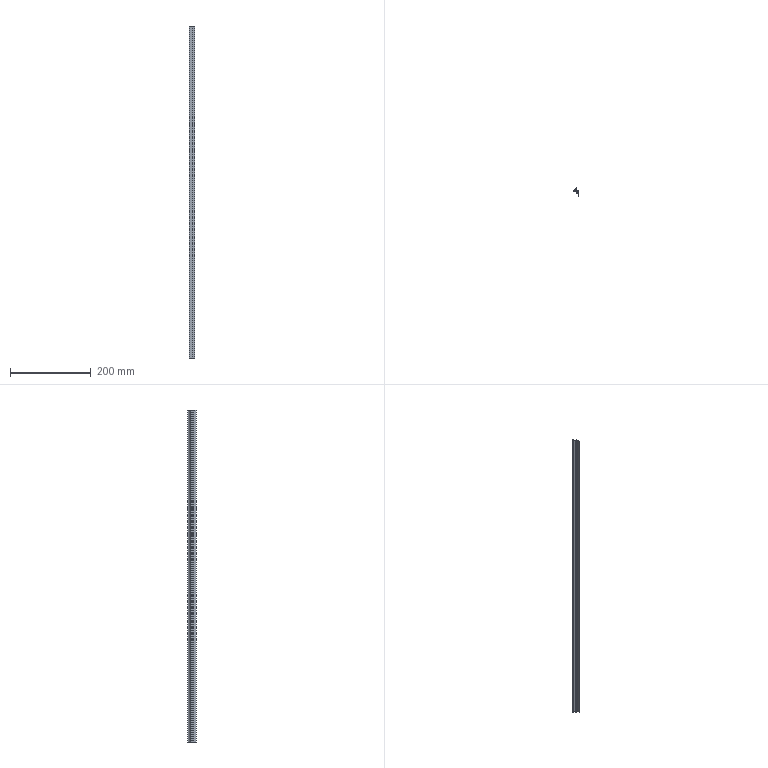Part | SolidWorks | features BaseBody 1, ICE 1, MoveFace 1 | 1 solid | 27 faces | box 14 x 20.3 x 820 mm | volume 41751 mm3 | plane 20 | cylinder 7 | commonest cylinder face diameters 0.387 x2 0.8 x2 0.4 x1 20 x1 22 x1
STEP:
#1=CARTESIAN_POINT('',(-5.304,-0.625,200.));
#2=VERTEX_POINT('',#1);
#3=CARTESIAN_POINT('',(-5.449,-0.8125,200.));
#4=VERTEX_POINT('',#3);
#5=CARTESIAN_POINT('',(-5.255,-0.8125,200.));
#6=DIRECTION('',(0.,0.,1.));
#7=DIRECTION('',(-1.,0.,0.));
#8=AXIS2_PLACEMENT_3D('',#5,#6,#7);
#9=CIRCLE('',#8,0.1937);
#10=EDGE_CURVE('',#2,#4,#9,.T.);
#11=ORIENTED_EDGE('',*,*,#10,.T.);
#12=CARTESIAN_POINT('',(-5.449,-0.8125,-620.));
#13=VERTEX_POINT('',#12);
#14=CARTESIAN_POINT('',(-5.449,-0.8125,230.));
#15=DIRECTION('',(0.,0.,-1.));
#16=VECTOR('',#15,1000.);
#17=LINE('',#14,#16);
#18=EDGE_CURVE('',#4,#13,#17,.T.);
#19=ORIENTED_EDGE('',*,*,#18,.T.);
#20=CARTESIAN_POINT('',(-5.304,-0.625,-620.));
#21=VERTEX_POINT('',#20);
#22=CARTESIAN_POINT('',(-5.255,-0.8125,-620.));
#23=DIRECTION('',(0.,0.,-1.));
#24=DIRECTION('',(1.,0.,0.));
#25=AXIS2_PLACEMENT_3D('',#22,#23,#24);
#26=CIRCLE('',#25,0.1937);
#27=EDGE_CURVE('',#13,#21,#26,.T.);
#28=ORIENTED_EDGE('',*,*,#27,.T.);
#29=CARTESIAN_POINT('',(-5.304,-0.625,230.));
#30=DIRECTION('',(0.,0.,-1.));
#31=VECTOR('',#30,1000.);
#32=LINE('',#29,#31);
#33=EDGE_CURVE('',#2,#21,#32,.T.);
#34=ORIENTED_EDGE('',*,*,#33,.F.);
#35=EDGE_LOOP('',(#11,#19,#28,#34));
#36=FACE_OUTER_BOUND('',#35,.T.);
#37=CARTESIAN_POINT('',(-5.255,-0.8125,230.));
#38=DIRECTION('',(0.,0.,-1.));
#39=DIRECTION('',(-1.,0.,0.));
#40=AXIS2_PLACEMENT_3D('',#37,#38,#39);
#41=CYLINDRICAL_SURFACE('',#40,0.1937);
#42=ADVANCED_FACE('',(#36),#41,.F.);
#43=CARTESIAN_POINT('',(5.,-1.,-620.));
#44=VERTEX_POINT('',#43);
#45=CARTESIAN_POINT('',(5.,-14.3,-620.));
#46=VERTEX_POINT('',#45);
#47=CARTESIAN_POINT('',(5.,29.623,-620.));
#48=DIRECTION('',(0.,-1.,0.));
#49=VECTOR('',#48,1000.);
#50=LINE('',#47,#49);
#51=EDGE_CURVE('',#44,#46,#50,.T.);
#52=ORIENTED_EDGE('',*,*,#51,.F.);
#53=CARTESIAN_POINT('',(5.,-1.,200.));
#54=VERTEX_POINT('',#53);
#55=CARTESIAN_POINT('',(5.,-1.,230.));
#56=DIRECTION('',(0.,0.,-1.));
#57=VECTOR('',#56,1000.);
#58=LINE('',#55,#57);
#59=EDGE_CURVE('',#54,#44,#58,.T.);
#60=ORIENTED_EDGE('',*,*,#59,.F.);
#61=CARTESIAN_POINT('',(5.,-14.3,200.));
#62=VERTEX_POINT('',#61);
#63=CARTESIAN_POINT('',(5.,-14.3,200.));
#64=DIRECTION('',(0.,1.,0.));
#65=VECTOR('',#64,1000.);
#66=LINE('',#63,#65);
#67=EDGE_CURVE('',#62,#54,#66,.T.);
#68=ORIENTED_EDGE('',*,*,#67,.F.);
#69=CARTESIAN_POINT('',(5.,-14.3,230.));
#70=DIRECTION('',(0.,0.,1.));
#71=VECTOR('',#70,1000.);
#72=LINE('',#69,#71);
#73=EDGE_CURVE('',#46,#62,#72,.T.);
#74=ORIENTED_EDGE('',*,*,#73,.F.);
#75=EDGE_LOOP('',(#52,#60,#68,#74));
#76=FACE_OUTER_BOUND('',#75,.T.);
#77=CARTESIAN_POINT('',(5.,-14.3,230.));
#78=DIRECTION('',(-1.,0.,0.));
#79=DIRECTION('',(0.,0.,1.));
#80=AXIS2_PLACEMENT_3D('',#77,#78,#79);
#81=PLANE('',#80);
#82=ADVANCED_FACE('',(#76),#81,.F.);
#83=CARTESIAN_POINT('',(-9.,-2.,-620.));
#84=VERTEX_POINT('',#83);
#85=CARTESIAN_POINT('',(-9.,-2.,200.));
#86=VERTEX_POINT('',#85);
#87=CARTESIAN_POINT('',(-9.,-2.,230.));
#88=DIRECTION('',(0.,0.,1.));
#89=VECTOR('',#88,1000.);
#90=LINE('',#87,#89);
#91=EDGE_CURVE('',#84,#86,#90,.T.);
#92=ORIENTED_EDGE('',*,*,#91,.F.);
#93=CARTESIAN_POINT('',(0.9,-2.,-620.));
#94=VERTEX_POINT('',#93);
#95=CARTESIAN_POINT('',(5.,-2.,-620.));
#96=DIRECTION('',(-1.,0.,0.));
#97=VECTOR('',#96,1000.);
#98=LINE('',#95,#97);
#99=EDGE_CURVE('',#94,#84,#98,.T.);
#100=ORIENTED_EDGE('',*,*,#99,.F.);
#101=CARTESIAN_POINT('',(0.9,-2.,200.));
#102=VERTEX_POINT('',#101);
#103=CARTESIAN_POINT('',(0.9,-2.,230.));
#104=DIRECTION('',(0.,0.,-1.));
#105=VECTOR('',#104,1000.);
#106=LINE('',#103,#105);
#107=EDGE_CURVE('',#102,#94,#106,.T.);
#108=ORIENTED_EDGE('',*,*,#107,.F.);
#109=CARTESIAN_POINT('',(5.,-2.,200.));
#110=DIRECTION('',(1.,0.,0.));
#111=VECTOR('',#110,1000.);
#112=LINE('',#109,#111);
#113=EDGE_CURVE('',#86,#102,#112,.T.);
#114=ORIENTED_EDGE('',*,*,#113,.F.);
#115=EDGE_LOOP('',(#92,#100,#108,#114));
#116=FACE_OUTER_BOUND('',#115,.T.);
#117=CARTESIAN_POINT('',(-9.,-2.,230.));
#118=DIRECTION('',(0.,1.,0.));
#119=DIRECTION('',(0.,0.,1.));
#120=AXIS2_PLACEMENT_3D('',#117,#118,#119);
#121=PLANE('',#120);
#122=ADVANCED_FACE('',(#116),#121,.F.);
#123=CARTESIAN_POINT('',(4.,-6.,200.));
#124=VERTEX_POINT('',#123);
#125=CARTESIAN_POINT('',(4.,-3.,200.));
#126=VERTEX_POINT('',#125);
#127=CARTESIAN_POINT('',(4.,29.623,200.));
#128=DIRECTION('',(0.,1.,0.));
#129=VECTOR('',#128,1000.);
#130=LINE('',#127,#129);
#131=EDGE_CURVE('',#124,#126,#130,.T.);
#132=ORIENTED_EDGE('',*,*,#131,.F.);
#133=CARTESIAN_POINT('',(1.,-6.,200.));
#134=VERTEX_POINT('',#133);
#135=CARTESIAN_POINT('',(5.,-6.,200.));
#136=DIRECTION('',(1.,0.,0.));
#137=VECTOR('',#136,1000.);
#138=LINE('',#135,#137);
#139=EDGE_CURVE('',#134,#124,#138,.T.);
#140=ORIENTED_EDGE('',*,*,#139,.F.);
#141=CARTESIAN_POINT('',(1.,-6.7,200.));
#142=VERTEX_POINT('',#141);
#143=CARTESIAN_POINT('',(1.,-6.,200.));
#144=DIRECTION('',(0.,-1.,0.));
#145=VECTOR('',#144,1000.);
#146=LINE('',#143,#145);
#147=EDGE_CURVE('',#134,#142,#146,.T.);
#148=ORIENTED_EDGE('',*,*,#147,.T.);
#149=CARTESIAN_POINT('',(-1.7,-6.7,200.));
#150=VERTEX_POINT('',#149);
#151=CARTESIAN_POINT('',(5.,-6.7,200.));
#152=DIRECTION('',(1.,0.,0.));
#153=VECTOR('',#152,1000.);
#154=LINE('',#151,#153);
#155=EDGE_CURVE('',#150,#142,#154,.T.);
#156=ORIENTED_EDGE('',*,*,#155,.F.);
#157=CARTESIAN_POINT('',(-1.7,-7.7,200.));
#158=VERTEX_POINT('',#157);
#159=CARTESIAN_POINT('',(-1.7,-6.7,200.));
#160=DIRECTION('',(0.,-1.,0.));
#161=VECTOR('',#160,1000.);
#162=LINE('',#159,#161);
#163=EDGE_CURVE('',#150,#158,#162,.T.);
#164=ORIENTED_EDGE('',*,*,#163,.T.);
#165=CARTESIAN_POINT('',(4.,-7.7,200.));
#166=VERTEX_POINT('',#165);
#167=CARTESIAN_POINT('',(5.,-7.7,200.));
#168=DIRECTION('',(-1.,0.,0.));
#169=VECTOR('',#168,1000.);
#170=LINE('',#167,#169);
#171=EDGE_CURVE('',#166,#158,#170,.T.);
#172=ORIENTED_EDGE('',*,*,#171,.F.);
#173=CARTESIAN_POINT('',(4.,-14.3,200.));
#174=VERTEX_POINT('',#173);
#175=CARTESIAN_POINT('',(4.,29.623,200.));
#176=DIRECTION('',(0.,1.,0.));
#177=VECTOR('',#176,1000.);
#178=LINE('',#175,#177);
#179=EDGE_CURVE('',#174,#166,#178,.T.);
#180=ORIENTED_EDGE('',*,*,#179,.F.);
#181=CARTESIAN_POINT('',(5.,-14.3,200.));
#182=DIRECTION('',(-1.,0.,0.));
#183=VECTOR('',#182,1000.);
#184=LINE('',#181,#183);
#185=EDGE_CURVE('',#62,#174,#184,.T.);
#186=ORIENTED_EDGE('',*,*,#185,.F.);
#187=ORIENTED_EDGE('',*,*,#67,.T.);
#188=CARTESIAN_POINT('',(-5.207,-1.,200.));
#189=VERTEX_POINT('',#188);
#190=CARTESIAN_POINT('',(5.,-1.,200.));
#191=DIRECTION('',(1.,0.,0.));
#192=VECTOR('',#191,1000.);
#193=LINE('',#190,#192);
#194=EDGE_CURVE('',#189,#54,#193,.T.);
#195=ORIENTED_EDGE('',*,*,#194,.F.);
#196=CARTESIAN_POINT('',(-5.255,-0.8125,200.));
#197=DIRECTION('',(0.,0.,1.));
#198=DIRECTION('',(-1.,0.,0.));
#199=AXIS2_PLACEMENT_3D('',#196,#197,#198);
#200=CIRCLE('',#199,0.1937);
#201=EDGE_CURVE('',#4,#189,#200,.T.);
#202=ORIENTED_EDGE('',*,*,#201,.F.);
#203=ORIENTED_EDGE('',*,*,#10,.F.);
#204=CARTESIAN_POINT('',(-1.368,3.063,200.));
#205=VERTEX_POINT('',#204);
#206=CARTESIAN_POINT('',(-10.628,9.,200.));
#207=DIRECTION('',(0.,0.,1.));
#208=DIRECTION('',(-1.,0.,0.));
#209=AXIS2_PLACEMENT_3D('',#206,#207,#208);
#210=CIRCLE('',#209,11.);
#211=EDGE_CURVE('',#2,#205,#210,.T.);
#212=ORIENTED_EDGE('',*,*,#211,.T.);
#213=CARTESIAN_POINT('',(-1.,2.955,200.));
#214=VERTEX_POINT('',#213);
#215=CARTESIAN_POINT('',(-1.2,2.955,200.));
#216=DIRECTION('',(0.,0.,1.));
#217=DIRECTION('',(-1.,0.,0.));
#218=AXIS2_PLACEMENT_3D('',#215,#216,#217);
#219=CIRCLE('',#218,0.2);
#220=EDGE_CURVE('',#214,#205,#219,.T.);
#221=ORIENTED_EDGE('',*,*,#220,.F.);
#222=CARTESIAN_POINT('',(-1.,1.5,200.));
#223=VERTEX_POINT('',#222);
#224=CARTESIAN_POINT('',(-1.,2.955,200.));
#225=DIRECTION('',(0.,1.,0.));
#226=VECTOR('',#225,1000.);
#227=LINE('',#224,#226);
#228=EDGE_CURVE('',#223,#214,#227,.T.);
#229=ORIENTED_EDGE('',*,*,#228,.F.);
#230=CARTESIAN_POINT('',(0.,1.5,200.));
#231=VERTEX_POINT('',#230);
#232=CARTESIAN_POINT('',(-1.,1.5,200.));
#233=DIRECTION('',(-1.,0.,0.));
#234=VECTOR('',#233,1000.);
#235=LINE('',#232,#234);
#236=EDGE_CURVE('',#231,#223,#235,.T.);
#237=ORIENTED_EDGE('',*,*,#236,.F.);
#238=CARTESIAN_POINT('',(0.,6.,200.));
#239=VERTEX_POINT('',#238);
#240=CARTESIAN_POINT('',(0.,1.5,200.));
#241=DIRECTION('',(0.,-1.,0.));
#242=VECTOR('',#241,1000.);
#243=LINE('',#240,#242);
#244=EDGE_CURVE('',#239,#231,#243,.T.);
#245=ORIENTED_EDGE('',*,*,#244,.F.);
#246=CARTESIAN_POINT('',(-0.8,6.,200.));
#247=VERTEX_POINT('',#246);
#248=CARTESIAN_POINT('',(0.,6.,200.));
#249=DIRECTION('',(1.,0.,0.));
#250=VECTOR('',#249,1000.);
#251=LINE('',#248,#250);
#252=EDGE_CURVE('',#247,#239,#251,.T.);
#253=ORIENTED_EDGE('',*,*,#252,.F.);
#254=CARTESIAN_POINT('',(-1.178,5.731,200.));
#255=VERTEX_POINT('',#254);
#256=CARTESIAN_POINT('',(-0.8,5.6,200.));
#257=DIRECTION('',(0.,0.,1.));
#258=DIRECTION('',(-1.,0.,0.));
#259=AXIS2_PLACEMENT_3D('',#256,#257,#258);
#260=CIRCLE('',#259,0.4);
#261=EDGE_CURVE('',#247,#255,#260,.T.);
#262=ORIENTED_EDGE('',*,*,#261,.T.);
#263=CARTESIAN_POINT('',(-8.678,-0.8077,200.));
#264=VERTEX_POINT('',#263);
#265=CARTESIAN_POINT('',(-10.628,9.,200.));
#266=DIRECTION('',(0.,0.,1.));
#267=DIRECTION('',(-1.,0.,0.));
#268=AXIS2_PLACEMENT_3D('',#265,#266,#267);
#269=CIRCLE('',#268,10.);
#270=EDGE_CURVE('',#264,#255,#269,.T.);
#271=ORIENTED_EDGE('',*,*,#270,.F.);
#272=CARTESIAN_POINT('',(-9.,-1.2,200.));
#273=VERTEX_POINT('',#272);
#274=CARTESIAN_POINT('',(-8.6,-1.2,200.));
#275=DIRECTION('',(0.,0.,1.));
#276=DIRECTION('',(-1.,0.,0.));
#277=AXIS2_PLACEMENT_3D('',#274,#275,#276);
#278=CIRCLE('',#277,0.4);
#279=EDGE_CURVE('',#264,#273,#278,.T.);
#280=ORIENTED_EDGE('',*,*,#279,.T.);
#281=CARTESIAN_POINT('',(-9.,8.,200.));
#282=DIRECTION('',(0.,-1.,0.));
#283=VECTOR('',#282,1000.);
#284=LINE('',#281,#283);
#285=EDGE_CURVE('',#273,#86,#284,.T.);
#286=ORIENTED_EDGE('',*,*,#285,.T.);
#287=ORIENTED_EDGE('',*,*,#113,.T.);
#288=CARTESIAN_POINT('',(0.9,-3.,200.));
#289=VERTEX_POINT('',#288);
#290=CARTESIAN_POINT('',(0.9,29.623,200.));
#291=DIRECTION('',(0.,1.,0.));
#292=VECTOR('',#291,1000.);
#293=LINE('',#290,#292);
#294=EDGE_CURVE('',#289,#102,#293,.T.);
#295=ORIENTED_EDGE('',*,*,#294,.F.);
#296=CARTESIAN_POINT('',(5.,-3.,200.));
#297=DIRECTION('',(-1.,0.,0.));
#298=VECTOR('',#297,1000.);
#299=LINE('',#296,#298);
#300=EDGE_CURVE('',#126,#289,#299,.T.);
#301=ORIENTED_EDGE('',*,*,#300,.F.);
#302=EDGE_LOOP('',(#132,#140,#148,#156,#164,#172,#180,#186,#187,#195,#202,#203,#212,#221,#229,#237,#245,#253,#262,#271,#280,#286,#287,#295,#301));
#303=FACE_OUTER_BOUND('',#302,.T.);
#304=CARTESIAN_POINT('',(5.,29.623,200.));
#305=DIRECTION('',(0.,0.,-1.));
#306=DIRECTION('',(-1.,0.,0.));
#307=AXIS2_PLACEMENT_3D('',#304,#305,#306);
#308=PLANE('',#307);
#309=ADVANCED_FACE('',(#303),#308,.F.);
#310=ORIENTED_EDGE('',*,*,#185,.T.);
#311=CARTESIAN_POINT('',(4.,-14.3,-620.));
#312=VERTEX_POINT('',#311);
#313=CARTESIAN_POINT('',(4.,-14.3,230.));
#314=DIRECTION('',(0.,0.,1.));
#315=VECTOR('',#314,1000.);
#316=LINE('',#313,#315);
#317=EDGE_CURVE('',#312,#174,#316,.T.);
#318=ORIENTED_EDGE('',*,*,#317,.F.);
#319=CARTESIAN_POINT('',(5.,-14.3,-620.));
#320=DIRECTION('',(-1.,0.,0.));
#321=VECTOR('',#320,1000.);
#322=LINE('',#319,#321);
#323=EDGE_CURVE('',#46,#312,#322,.T.);
#324=ORIENTED_EDGE('',*,*,#323,.F.);
#325=ORIENTED_EDGE('',*,*,#73,.T.);
#326=EDGE_LOOP('',(#310,#318,#324,#325));
#327=FACE_OUTER_BOUND('',#326,.T.);
#328=CARTESIAN_POINT('',(4.,-14.3,230.));
#329=DIRECTION('',(0.,1.,0.));
#330=DIRECTION('',(0.,0.,1.));
#331=AXIS2_PLACEMENT_3D('',#328,#329,#330);
#332=PLANE('',#331);
#333=ADVANCED_FACE('',(#327),#332,.F.);
#334=ORIENTED_EDGE('',*,*,#51,.T.);
#335=ORIENTED_EDGE('',*,*,#323,.T.);
#336=CARTESIAN_POINT('',(4.,-7.7,-620.));
#337=VERTEX_POINT('',#336);
#338=CARTESIAN_POINT('',(4.,-7.7,-620.));
#339=DIRECTION('',(0.,-1.,0.));
#340=VECTOR('',#339,1000.);
#341=LINE('',#338,#340);
#342=EDGE_CURVE('',#337,#312,#341,.T.);
#343=ORIENTED_EDGE('',*,*,#342,.F.);
#344=CARTESIAN_POINT('',(-1.7,-7.7,-620.));
#345=VERTEX_POINT('',#344);
#346=CARTESIAN_POINT('',(-1.7,-7.7,-620.));
#347=DIRECTION('',(1.,0.,0.));
#348=VECTOR('',#347,1000.);
#349=LINE('',#346,#348);
#350=EDGE_CURVE('',#345,#337,#349,.T.);
#351=ORIENTED_EDGE('',*,*,#350,.F.);
#352=CARTESIAN_POINT('',(-1.7,-6.7,-620.));
#353=VERTEX_POINT('',#352);
#354=CARTESIAN_POINT('',(-1.7,29.623,-620.));
#355=DIRECTION('',(0.,1.,0.));
#356=VECTOR('',#355,1000.);
#357=LINE('',#354,#356);
#358=EDGE_CURVE('',#345,#353,#357,.T.);
#359=ORIENTED_EDGE('',*,*,#358,.T.);
#360=CARTESIAN_POINT('',(1.,-6.7,-620.));
#361=VERTEX_POINT('',#360);
#362=CARTESIAN_POINT('',(1.,-6.7,-620.));
#363=DIRECTION('',(-1.,0.,0.));
#364=VECTOR('',#363,1000.);
#365=LINE('',#362,#364);
#366=EDGE_CURVE('',#361,#353,#365,.T.);
#367=ORIENTED_EDGE('',*,*,#366,.F.);
#368=CARTESIAN_POINT('',(1.,-6.,-620.));
#369=VERTEX_POINT('',#368);
#370=CARTESIAN_POINT('',(1.,29.623,-620.));
#371=DIRECTION('',(0.,1.,0.));
#372=VECTOR('',#371,1000.);
#373=LINE('',#370,#372);
#374=EDGE_CURVE('',#361,#369,#373,.T.);
#375=ORIENTED_EDGE('',*,*,#374,.T.);
#376=CARTESIAN_POINT('',(4.,-6.,-620.));
#377=VERTEX_POINT('',#376);
#378=CARTESIAN_POINT('',(4.,-6.,-620.));
#379=DIRECTION('',(-1.,0.,0.));
#380=VECTOR('',#379,1000.);
#381=LINE('',#378,#380);
#382=EDGE_CURVE('',#377,#369,#381,.T.);
#383=ORIENTED_EDGE('',*,*,#382,.F.);
#384=CARTESIAN_POINT('',(4.,-3.,-620.));
#385=VERTEX_POINT('',#384);
#386=CARTESIAN_POINT('',(4.,-3.,-620.));
#387=DIRECTION('',(0.,-1.,0.));
#388=VECTOR('',#387,1000.);
#389=LINE('',#386,#388);
#390=EDGE_CURVE('',#385,#377,#389,.T.);
#391=ORIENTED_EDGE('',*,*,#390,.F.);
#392=CARTESIAN_POINT('',(0.9,-3.,-620.));
#393=VERTEX_POINT('',#392);
#394=CARTESIAN_POINT('',(0.9,-3.,-620.));
#395=DIRECTION('',(1.,0.,0.));
#396=VECTOR('',#395,1000.);
#397=LINE('',#394,#396);
#398=EDGE_CURVE('',#393,#385,#397,.T.);
#399=ORIENTED_EDGE('',*,*,#398,.F.);
#400=CARTESIAN_POINT('',(0.9,-2.,-620.));
#401=DIRECTION('',(0.,-1.,0.));
#402=VECTOR('',#401,1000.);
#403=LINE('',#400,#402);
#404=EDGE_CURVE('',#94,#393,#403,.T.);
#405=ORIENTED_EDGE('',*,*,#404,.F.);
#406=ORIENTED_EDGE('',*,*,#99,.T.);
#407=CARTESIAN_POINT('',(-9.,-1.2,-620.));
#408=VERTEX_POINT('',#407);
#409=CARTESIAN_POINT('',(-9.,-1.2,-620.));
#410=DIRECTION('',(0.,-1.,0.));
#411=VECTOR('',#410,1000.);
#412=LINE('',#409,#411);
#413=EDGE_CURVE('',#408,#84,#412,.T.);
#414=ORIENTED_EDGE('',*,*,#413,.F.);
#415=CARTESIAN_POINT('',(-8.678,-0.8077,-620.));
#416=VERTEX_POINT('',#415);
#417=CARTESIAN_POINT('',(-8.6,-1.2,-620.));
#418=DIRECTION('',(0.,0.,-1.));
#419=DIRECTION('',(1.,0.,0.));
#420=AXIS2_PLACEMENT_3D('',#417,#418,#419);
#421=CIRCLE('',#420,0.4);
#422=EDGE_CURVE('',#408,#416,#421,.T.);
#423=ORIENTED_EDGE('',*,*,#422,.T.);
#424=CARTESIAN_POINT('',(-1.178,5.731,-620.));
#425=VERTEX_POINT('',#424);
#426=CARTESIAN_POINT('',(-10.628,9.,-620.));
#427=DIRECTION('',(0.,0.,-1.));
#428=DIRECTION('',(1.,0.,0.));
#429=AXIS2_PLACEMENT_3D('',#426,#427,#428);
#430=CIRCLE('',#429,10.);
#431=EDGE_CURVE('',#425,#416,#430,.T.);
#432=ORIENTED_EDGE('',*,*,#431,.F.);
#433=CARTESIAN_POINT('',(-0.8,6.,-620.));
#434=VERTEX_POINT('',#433);
#435=CARTESIAN_POINT('',(-0.8,5.6,-620.));
#436=DIRECTION('',(0.,0.,-1.));
#437=DIRECTION('',(1.,0.,0.));
#438=AXIS2_PLACEMENT_3D('',#435,#436,#437);
#439=CIRCLE('',#438,0.4);
#440=EDGE_CURVE('',#425,#434,#439,.T.);
#441=ORIENTED_EDGE('',*,*,#440,.T.);
#442=CARTESIAN_POINT('',(0.,6.,-620.));
#443=VERTEX_POINT('',#442);
#444=CARTESIAN_POINT('',(0.,6.,-620.));
#445=DIRECTION('',(-1.,0.,0.));
#446=VECTOR('',#445,1000.);
#447=LINE('',#444,#446);
#448=EDGE_CURVE('',#443,#434,#447,.T.);
#449=ORIENTED_EDGE('',*,*,#448,.F.);
#450=CARTESIAN_POINT('',(0.,1.5,-620.));
#451=VERTEX_POINT('',#450);
#452=CARTESIAN_POINT('',(0.,1.5,-620.));
#453=DIRECTION('',(0.,1.,0.));
#454=VECTOR('',#453,1000.);
#455=LINE('',#452,#454);
#456=EDGE_CURVE('',#451,#443,#455,.T.);
#457=ORIENTED_EDGE('',*,*,#456,.F.);
#458=CARTESIAN_POINT('',(-1.,1.5,-620.));
#459=VERTEX_POINT('',#458);
#460=CARTESIAN_POINT('',(-1.,1.5,-620.));
#461=DIRECTION('',(1.,0.,0.));
#462=VECTOR('',#461,1000.);
#463=LINE('',#460,#462);
#464=EDGE_CURVE('',#459,#451,#463,.T.);
#465=ORIENTED_EDGE('',*,*,#464,.F.);
#466=CARTESIAN_POINT('',(-1.,2.955,-620.));
#467=VERTEX_POINT('',#466);
#468=CARTESIAN_POINT('',(-1.,2.955,-620.));
#469=DIRECTION('',(0.,-1.,0.));
#470=VECTOR('',#469,1000.);
#471=LINE('',#468,#470);
#472=EDGE_CURVE('',#467,#459,#471,.T.);
#473=ORIENTED_EDGE('',*,*,#472,.F.);
#474=CARTESIAN_POINT('',(-1.368,3.063,-620.));
#475=VERTEX_POINT('',#474);
#476=CARTESIAN_POINT('',(-1.2,2.955,-620.));
#477=DIRECTION('',(0.,0.,-1.));
#478=DIRECTION('',(1.,0.,0.));
#479=AXIS2_PLACEMENT_3D('',#476,#477,#478);
#480=CIRCLE('',#479,0.2);
#481=EDGE_CURVE('',#475,#467,#480,.T.);
#482=ORIENTED_EDGE('',*,*,#481,.F.);
#483=CARTESIAN_POINT('',(-10.628,9.,-620.));
#484=DIRECTION('',(0.,0.,-1.));
#485=DIRECTION('',(1.,0.,0.));
#486=AXIS2_PLACEMENT_3D('',#483,#484,#485);
#487=CIRCLE('',#486,11.);
#488=EDGE_CURVE('',#475,#21,#487,.T.);
#489=ORIENTED_EDGE('',*,*,#488,.T.);
#490=ORIENTED_EDGE('',*,*,#27,.F.);
#491=CARTESIAN_POINT('',(-5.207,-1.,-620.));
#492=VERTEX_POINT('',#491);
#493=CARTESIAN_POINT('',(-5.255,-0.8125,-620.));
#494=DIRECTION('',(0.,0.,-1.));
#495=DIRECTION('',(1.,0.,0.));
#496=AXIS2_PLACEMENT_3D('',#493,#494,#495);
#497=CIRCLE('',#496,0.1937);
#498=EDGE_CURVE('',#492,#13,#497,.T.);
#499=ORIENTED_EDGE('',*,*,#498,.F.);
#500=CARTESIAN_POINT('',(5.,-1.,-620.));
#501=DIRECTION('',(-1.,0.,0.));
#502=VECTOR('',#501,1000.);
#503=LINE('',#500,#502);
#504=EDGE_CURVE('',#44,#492,#503,.T.);
#505=ORIENTED_EDGE('',*,*,#504,.F.);
#506=EDGE_LOOP('',(#334,#335,#343,#351,#359,#367,#375,#383,#391,#399,#405,#406,#414,#423,#432,#441,#449,#457,#465,#473,#482,#489,#490,#499,#505));
#507=FACE_OUTER_BOUND('',#506,.T.);
#508=CARTESIAN_POINT('',(5.,29.623,-620.));
#509=DIRECTION('',(0.,0.,1.));
#510=DIRECTION('',(1.,0.,0.));
#511=AXIS2_PLACEMENT_3D('',#508,#509,#510);
#512=PLANE('',#511);
#513=ADVANCED_FACE('',(#507),#512,.F.);
#514=ORIENTED_EDGE('',*,*,#59,.T.);
#515=ORIENTED_EDGE('',*,*,#504,.T.);
#516=CARTESIAN_POINT('',(-5.207,-1.,230.));
#517=DIRECTION('',(0.,0.,-1.));
#518=VECTOR('',#517,1000.);
#519=LINE('',#516,#518);
#520=EDGE_CURVE('',#189,#492,#519,.T.);
#521=ORIENTED_EDGE('',*,*,#520,.F.);
#522=ORIENTED_EDGE('',*,*,#194,.T.);
#523=EDGE_LOOP('',(#514,#515,#521,#522));
#524=FACE_OUTER_BOUND('',#523,.T.);
#525=CARTESIAN_POINT('',(5.,-1.,230.));
#526=DIRECTION('',(0.,-1.,0.));
#527=DIRECTION('',(0.,0.,-1.));
#528=AXIS2_PLACEMENT_3D('',#525,#526,#527);
#529=PLANE('',#528);
#530=ADVANCED_FACE('',(#524),#529,.F.);
#531=CARTESIAN_POINT('',(-9.,-1.2,230.));
#532=DIRECTION('',(0.,0.,1.));
#533=VECTOR('',#532,1000.);
#534=LINE('',#531,#533);
#535=EDGE_CURVE('',#408,#273,#534,.T.);
#536=ORIENTED_EDGE('',*,*,#535,.F.);
#537=ORIENTED_EDGE('',*,*,#413,.T.);
#538=ORIENTED_EDGE('',*,*,#91,.T.);
#539=ORIENTED_EDGE('',*,*,#285,.F.);
#540=EDGE_LOOP('',(#536,#537,#538,#539));
#541=FACE_OUTER_BOUND('',#540,.T.);
#542=CARTESIAN_POINT('',(-9.,-1.2,230.));
#543=DIRECTION('',(1.,0.,0.));
#544=DIRECTION('',(0.,0.,-1.));
#545=AXIS2_PLACEMENT_3D('',#542,#543,#544);
#546=PLANE('',#545);
#547=ADVANCED_FACE('',(#541),#546,.F.);
#548=ORIENTED_EDGE('',*,*,#294,.T.);
#549=ORIENTED_EDGE('',*,*,#107,.T.);
#550=ORIENTED_EDGE('',*,*,#404,.T.);
#551=CARTESIAN_POINT('',(0.9,-3.,230.));
#552=DIRECTION('',(0.,0.,-1.));
#553=VECTOR('',#552,1000.);
#554=LINE('',#551,#553);
#555=EDGE_CURVE('',#289,#393,#554,.T.);
#556=ORIENTED_EDGE('',*,*,#555,.F.);
#557=EDGE_LOOP('',(#548,#549,#550,#556));
#558=FACE_OUTER_BOUND('',#557,.T.);
#559=CARTESIAN_POINT('',(0.9,-2.,230.));
#560=DIRECTION('',(1.,0.,0.));
#561=DIRECTION('',(0.,0.,-1.));
#562=AXIS2_PLACEMENT_3D('',#559,#560,#561);
#563=PLANE('',#562);
#564=ADVANCED_FACE('',(#558),#563,.F.);
#565=ORIENTED_EDGE('',*,*,#300,.T.);
#566=ORIENTED_EDGE('',*,*,#555,.T.);
#567=ORIENTED_EDGE('',*,*,#398,.T.);
#568=CARTESIAN_POINT('',(4.,-3.,230.));
#569=DIRECTION('',(0.,0.,-1.));
#570=VECTOR('',#569,1000.);
#571=LINE('',#568,#570);
#572=EDGE_CURVE('',#126,#385,#571,.T.);
#573=ORIENTED_EDGE('',*,*,#572,.F.);
#574=EDGE_LOOP('',(#565,#566,#567,#573));
#575=FACE_OUTER_BOUND('',#574,.T.);
#576=CARTESIAN_POINT('',(0.9,-3.,230.));
#577=DIRECTION('',(0.,1.,0.));
#578=DIRECTION('',(0.,0.,1.));
#579=AXIS2_PLACEMENT_3D('',#576,#577,#578);
#580=PLANE('',#579);
#581=ADVANCED_FACE('',(#575),#580,.F.);
#582=ORIENTED_EDGE('',*,*,#131,.T.);
#583=ORIENTED_EDGE('',*,*,#572,.T.);
#584=ORIENTED_EDGE('',*,*,#390,.T.);
#585=CARTESIAN_POINT('',(4.,-6.,230.));
#586=DIRECTION('',(0.,0.,-1.));
#587=VECTOR('',#586,1000.);
#588=LINE('',#585,#587);
#589=EDGE_CURVE('',#124,#377,#588,.T.);
#590=ORIENTED_EDGE('',*,*,#589,.F.);
#591=EDGE_LOOP('',(#582,#583,#584,#590));
#592=FACE_OUTER_BOUND('',#591,.T.);
#593=CARTESIAN_POINT('',(4.,-3.,230.));
#594=DIRECTION('',(1.,0.,0.));
#595=DIRECTION('',(0.,0.,-1.));
#596=AXIS2_PLACEMENT_3D('',#593,#594,#595);
#597=PLANE('',#596);
#598=ADVANCED_FACE('',(#592),#597,.F.);
#599=ORIENTED_EDGE('',*,*,#139,.T.);
#600=ORIENTED_EDGE('',*,*,#589,.T.);
#601=ORIENTED_EDGE('',*,*,#382,.T.);
#602=CARTESIAN_POINT('',(1.,-6.,230.));
#603=DIRECTION('',(0.,0.,-1.));
#604=VECTOR('',#603,1000.);
#605=LINE('',#602,#604);
#606=EDGE_CURVE('',#134,#369,#605,.T.);
#607=ORIENTED_EDGE('',*,*,#606,.F.);
#608=EDGE_LOOP('',(#599,#600,#601,#607));
#609=FACE_OUTER_BOUND('',#608,.T.);
#610=CARTESIAN_POINT('',(4.,-6.,230.));
#611=DIRECTION('',(0.,-1.,0.));
#612=DIRECTION('',(0.,0.,-1.));
#613=AXIS2_PLACEMENT_3D('',#610,#611,#612);
#614=PLANE('',#613);
#615=ADVANCED_FACE('',(#609),#614,.F.);
#616=ORIENTED_EDGE('',*,*,#155,.T.);
#617=CARTESIAN_POINT('',(1.,-6.7,230.));
#618=DIRECTION('',(0.,0.,1.));
#619=VECTOR('',#618,1000.);
#620=LINE('',#617,#619);
#621=EDGE_CURVE('',#361,#142,#620,.T.);
#622=ORIENTED_EDGE('',*,*,#621,.F.);
#623=ORIENTED_EDGE('',*,*,#366,.T.);
#624=CARTESIAN_POINT('',(-1.7,-6.7,230.));
#625=DIRECTION('',(0.,0.,-1.));
#626=VECTOR('',#625,1000.);
#627=LINE('',#624,#626);
#628=EDGE_CURVE('',#150,#353,#627,.T.);
#629=ORIENTED_EDGE('',*,*,#628,.F.);
#630=EDGE_LOOP('',(#616,#622,#623,#629));
#631=FACE_OUTER_BOUND('',#630,.T.);
#632=CARTESIAN_POINT('',(1.,-6.7,230.));
#633=DIRECTION('',(0.,-1.,0.));
#634=DIRECTION('',(0.,0.,-1.));
#635=AXIS2_PLACEMENT_3D('',#632,#633,#634);
#636=PLANE('',#635);
#637=ADVANCED_FACE('',(#631),#636,.F.);
#638=ORIENTED_EDGE('',*,*,#171,.T.);
#639=CARTESIAN_POINT('',(-1.7,-7.7,230.));
#640=DIRECTION('',(0.,0.,1.));
#641=VECTOR('',#640,1000.);
#642=LINE('',#639,#641);
#643=EDGE_CURVE('',#345,#158,#642,.T.);
#644=ORIENTED_EDGE('',*,*,#643,.F.);
#645=ORIENTED_EDGE('',*,*,#350,.T.);
#646=CARTESIAN_POINT('',(4.,-7.7,230.));
#647=DIRECTION('',(0.,0.,-1.));
#648=VECTOR('',#647,1000.);
#649=LINE('',#646,#648);
#650=EDGE_CURVE('',#166,#337,#649,.T.);
#651=ORIENTED_EDGE('',*,*,#650,.F.);
#652=EDGE_LOOP('',(#638,#644,#645,#651));
#653=FACE_OUTER_BOUND('',#652,.T.);
#654=CARTESIAN_POINT('',(-1.7,-7.7,230.));
#655=DIRECTION('',(0.,1.,0.));
#656=DIRECTION('',(0.,0.,1.));
#657=AXIS2_PLACEMENT_3D('',#654,#655,#656);
#658=PLANE('',#657);
#659=ADVANCED_FACE('',(#653),#658,.F.);
#660=ORIENTED_EDGE('',*,*,#179,.T.);
#661=ORIENTED_EDGE('',*,*,#650,.T.);
#662=ORIENTED_EDGE('',*,*,#342,.T.);
#663=ORIENTED_EDGE('',*,*,#317,.T.);
#664=EDGE_LOOP('',(#660,#661,#662,#663));
#665=FACE_OUTER_BOUND('',#664,.T.);
#666=CARTESIAN_POINT('',(4.,-7.7,230.));
#667=DIRECTION('',(1.,0.,0.));
#668=DIRECTION('',(0.,0.,-1.));
#669=AXIS2_PLACEMENT_3D('',#666,#667,#668);
#670=PLANE('',#669);
#671=ADVANCED_FACE('',(#665),#670,.F.);
#672=ORIENTED_EDGE('',*,*,#18,.F.);
#673=ORIENTED_EDGE('',*,*,#201,.T.);
#674=ORIENTED_EDGE('',*,*,#520,.T.);
#675=ORIENTED_EDGE('',*,*,#498,.T.);
#676=EDGE_LOOP('',(#672,#673,#674,#675));
#677=FACE_OUTER_BOUND('',#676,.T.);
#678=CARTESIAN_POINT('',(-5.255,-0.8125,230.));
#679=DIRECTION('',(0.,0.,-1.));
#680=DIRECTION('',(-1.,0.,0.));
#681=AXIS2_PLACEMENT_3D('',#678,#679,#680);
#682=CYLINDRICAL_SURFACE('',#681,0.1937);
#683=ADVANCED_FACE('',(#677),#682,.F.);
#684=CARTESIAN_POINT('',(-1.,2.955,230.));
#685=DIRECTION('',(0.,0.,1.));
#686=VECTOR('',#685,1000.);
#687=LINE('',#684,#686);
#688=EDGE_CURVE('',#467,#214,#687,.T.);
#689=ORIENTED_EDGE('',*,*,#688,.F.);
#690=ORIENTED_EDGE('',*,*,#472,.T.);
#691=CARTESIAN_POINT('',(-1.,1.5,230.));
#692=DIRECTION('',(0.,0.,-1.));
#693=VECTOR('',#692,1000.);
#694=LINE('',#691,#693);
#695=EDGE_CURVE('',#223,#459,#694,.T.);
#696=ORIENTED_EDGE('',*,*,#695,.F.);
#697=ORIENTED_EDGE('',*,*,#228,.T.);
#698=EDGE_LOOP('',(#689,#690,#696,#697));
#699=FACE_OUTER_BOUND('',#698,.T.);
#700=CARTESIAN_POINT('',(-1.,2.955,230.));
#701=DIRECTION('',(1.,0.,0.));
#702=DIRECTION('',(0.,0.,-1.));
#703=AXIS2_PLACEMENT_3D('',#700,#701,#702);
#704=PLANE('',#703);
#705=ADVANCED_FACE('',(#699),#704,.F.);
#706=ORIENTED_EDGE('',*,*,#488,.F.);
#707=CARTESIAN_POINT('',(-1.368,3.063,230.));
#708=DIRECTION('',(0.,0.,1.));
#709=VECTOR('',#708,1000.);
#710=LINE('',#707,#709);
#711=EDGE_CURVE('',#475,#205,#710,.T.);
#712=ORIENTED_EDGE('',*,*,#711,.T.);
#713=ORIENTED_EDGE('',*,*,#211,.F.);
#714=ORIENTED_EDGE('',*,*,#33,.T.);
#715=EDGE_LOOP('',(#706,#712,#713,#714));
#716=FACE_OUTER_BOUND('',#715,.T.);
#717=CARTESIAN_POINT('',(-10.628,9.,230.));
#718=DIRECTION('',(0.,0.,-1.));
#719=DIRECTION('',(-1.,0.,0.));
#720=AXIS2_PLACEMENT_3D('',#717,#718,#719);
#721=CYLINDRICAL_SURFACE('',#720,11.);
#722=ADVANCED_FACE('',(#716),#721,.T.);
#723=CARTESIAN_POINT('',(-1.178,5.731,230.));
#724=DIRECTION('',(0.,0.,1.));
#725=VECTOR('',#724,1000.);
#726=LINE('',#723,#725);
#727=EDGE_CURVE('',#425,#255,#726,.T.);
#728=ORIENTED_EDGE('',*,*,#727,.F.);
#729=ORIENTED_EDGE('',*,*,#431,.T.);
#730=CARTESIAN_POINT('',(-8.678,-0.8077,230.));
#731=DIRECTION('',(0.,0.,-1.));
#732=VECTOR('',#731,1000.);
#733=LINE('',#730,#732);
#734=EDGE_CURVE('',#264,#416,#733,.T.);
#735=ORIENTED_EDGE('',*,*,#734,.F.);
#736=ORIENTED_EDGE('',*,*,#270,.T.);
#737=EDGE_LOOP('',(#728,#729,#735,#736));
#738=FACE_OUTER_BOUND('',#737,.T.);
#739=CARTESIAN_POINT('',(-10.628,9.,230.));
#740=DIRECTION('',(0.,0.,-1.));
#741=DIRECTION('',(-1.,0.,0.));
#742=AXIS2_PLACEMENT_3D('',#739,#740,#741);
#743=CYLINDRICAL_SURFACE('',#742,10.);
#744=ADVANCED_FACE('',(#738),#743,.F.);
#745=CARTESIAN_POINT('',(0.,1.5,230.));
#746=DIRECTION('',(0.,0.,1.));
#747=VECTOR('',#746,1000.);
#748=LINE('',#745,#747);
#749=EDGE_CURVE('',#451,#231,#748,.T.);
#750=ORIENTED_EDGE('',*,*,#749,.F.);
#751=ORIENTED_EDGE('',*,*,#456,.T.);
#752=CARTESIAN_POINT('',(0.,6.,230.));
#753=DIRECTION('',(0.,0.,-1.));
#754=VECTOR('',#753,1000.);
#755=LINE('',#752,#754);
#756=EDGE_CURVE('',#239,#443,#755,.T.);
#757=ORIENTED_EDGE('',*,*,#756,.F.);
#758=ORIENTED_EDGE('',*,*,#244,.T.);
#759=EDGE_LOOP('',(#750,#751,#757,#758));
#760=FACE_OUTER_BOUND('',#759,.T.);
#761=CARTESIAN_POINT('',(0.,1.5,230.));
#762=DIRECTION('',(-1.,0.,0.));
#763=DIRECTION('',(0.,0.,1.));
#764=AXIS2_PLACEMENT_3D('',#761,#762,#763);
#765=PLANE('',#764);
#766=ADVANCED_FACE('',(#760),#765,.F.);
#767=ORIENTED_EDGE('',*,*,#422,.F.);
#768=ORIENTED_EDGE('',*,*,#535,.T.);
#769=ORIENTED_EDGE('',*,*,#279,.F.);
#770=ORIENTED_EDGE('',*,*,#734,.T.);
#771=EDGE_LOOP('',(#767,#768,#769,#770));
#772=FACE_OUTER_BOUND('',#771,.T.);
#773=CARTESIAN_POINT('',(-8.6,-1.2,230.));
#774=DIRECTION('',(0.,0.,-1.));
#775=DIRECTION('',(-1.,0.,0.));
#776=AXIS2_PLACEMENT_3D('',#773,#774,#775);
#777=CYLINDRICAL_SURFACE('',#776,0.4);
#778=ADVANCED_FACE('',(#772),#777,.T.);
#779=ORIENTED_EDGE('',*,*,#147,.F.);
#780=ORIENTED_EDGE('',*,*,#606,.T.);
#781=ORIENTED_EDGE('',*,*,#374,.F.);
#782=ORIENTED_EDGE('',*,*,#621,.T.);
#783=EDGE_LOOP('',(#779,#780,#781,#782));
#784=FACE_OUTER_BOUND('',#783,.T.);
#785=CARTESIAN_POINT('',(1.,-6.,230.));
#786=DIRECTION('',(1.,0.,0.));
#787=DIRECTION('',(0.,0.,-1.));
#788=AXIS2_PLACEMENT_3D('',#785,#786,#787);
#789=PLANE('',#788);
#790=ADVANCED_FACE('',(#784),#789,.F.);
#791=ORIENTED_EDGE('',*,*,#163,.F.);
#792=ORIENTED_EDGE('',*,*,#628,.T.);
#793=ORIENTED_EDGE('',*,*,#358,.F.);
#794=ORIENTED_EDGE('',*,*,#643,.T.);
#795=EDGE_LOOP('',(#791,#792,#793,#794));
#796=FACE_OUTER_BOUND('',#795,.T.);
#797=CARTESIAN_POINT('',(-1.7,-6.7,230.));
#798=DIRECTION('',(1.,0.,0.));
#799=DIRECTION('',(0.,0.,-1.));
#800=AXIS2_PLACEMENT_3D('',#797,#798,#799);
#801=PLANE('',#800);
#802=ADVANCED_FACE('',(#796),#801,.F.);
#803=ORIENTED_EDGE('',*,*,#711,.F.);
#804=ORIENTED_EDGE('',*,*,#481,.T.);
#805=ORIENTED_EDGE('',*,*,#688,.T.);
#806=ORIENTED_EDGE('',*,*,#220,.T.);
#807=EDGE_LOOP('',(#803,#804,#805,#806));
#808=FACE_OUTER_BOUND('',#807,.T.);
#809=CARTESIAN_POINT('',(-1.2,2.955,230.));
#810=DIRECTION('',(0.,0.,-1.));
#811=DIRECTION('',(-1.,0.,0.));
#812=AXIS2_PLACEMENT_3D('',#809,#810,#811);
#813=CYLINDRICAL_SURFACE('',#812,0.2);
#814=ADVANCED_FACE('',(#808),#813,.F.);
#815=ORIENTED_EDGE('',*,*,#695,.T.);
#816=ORIENTED_EDGE('',*,*,#464,.T.);
#817=ORIENTED_EDGE('',*,*,#749,.T.);
#818=ORIENTED_EDGE('',*,*,#236,.T.);
#819=EDGE_LOOP('',(#815,#816,#817,#818));
#820=FACE_OUTER_BOUND('',#819,.T.);
#821=CARTESIAN_POINT('',(-1.,1.5,230.));
#822=DIRECTION('',(0.,1.,0.));
#823=DIRECTION('',(0.,0.,1.));
#824=AXIS2_PLACEMENT_3D('',#821,#822,#823);
#825=PLANE('',#824);
#826=ADVANCED_FACE('',(#820),#825,.F.);
#827=ORIENTED_EDGE('',*,*,#440,.F.);
#828=ORIENTED_EDGE('',*,*,#727,.T.);
#829=ORIENTED_EDGE('',*,*,#261,.F.);
#830=CARTESIAN_POINT('',(-0.8,6.,230.));
#831=DIRECTION('',(0.,0.,-1.));
#832=VECTOR('',#831,1000.);
#833=LINE('',#830,#832);
#834=EDGE_CURVE('',#247,#434,#833,.T.);
#835=ORIENTED_EDGE('',*,*,#834,.T.);
#836=EDGE_LOOP('',(#827,#828,#829,#835));
#837=FACE_OUTER_BOUND('',#836,.T.);
#838=CARTESIAN_POINT('',(-0.8,5.6,230.));
#839=DIRECTION('',(0.,0.,-1.));
#840=DIRECTION('',(-1.,0.,0.));
#841=AXIS2_PLACEMENT_3D('',#838,#839,#840);
#842=CYLINDRICAL_SURFACE('',#841,0.4);
#843=ADVANCED_FACE('',(#837),#842,.T.);
#844=ORIENTED_EDGE('',*,*,#756,.T.);
#845=ORIENTED_EDGE('',*,*,#448,.T.);
#846=ORIENTED_EDGE('',*,*,#834,.F.);
#847=ORIENTED_EDGE('',*,*,#252,.T.);
#848=EDGE_LOOP('',(#844,#845,#846,#847));
#849=FACE_OUTER_BOUND('',#848,.T.);
#850=CARTESIAN_POINT('',(0.,6.,230.));
#851=DIRECTION('',(0.,-1.,0.));
#852=DIRECTION('',(0.,0.,-1.));
#853=AXIS2_PLACEMENT_3D('',#850,#851,#852);
#854=PLANE('',#853);
#855=ADVANCED_FACE('',(#849),#854,.F.);
#856=CLOSED_SHELL('',(#42,#82,#122,#309,#333,#513,#530,#547,#564,#581,#598,#615,#637,#659,#671,#683,#705,#722,#744,#766,#778,#790,#802,#814,#826,#843,#855));
#857=MANIFOLD_SOLID_BREP('',#856);
#858=CARTESIAN_POINT('',(0.,0.,0.));
#859=DIRECTION('',(0.,0.,1.));
#860=DIRECTION('',(1.,0.,0.));
#861=AXIS2_PLACEMENT_3D('',#858,#859,#860);
#862=(LENGTH_UNIT()NAMED_UNIT(*)SI_UNIT(.MILLI.,.METRE.));
#863=UNCERTAINTY_MEASURE_WITH_UNIT(LENGTH_MEASURE(0.00001),#862,'','');
#864=(NAMED_UNIT(*)PLANE_ANGLE_UNIT()SI_UNIT($,.RADIAN.));
#865=(NAMED_UNIT(*)SI_UNIT($,.STERADIAN.)SOLID_ANGLE_UNIT());
#866=(GEOMETRIC_REPRESENTATION_CONTEXT(3)GLOBAL_UNCERTAINTY_ASSIGNED_CONTEXT((#863))GLOBAL_UNIT_ASSIGNED_CONTEXT((#862,#864,#865))REPRESENTATION_CONTEXT('',''));
#867=ADVANCED_BREP_SHAPE_REPRESENTATION('',(#857,#861),#866);